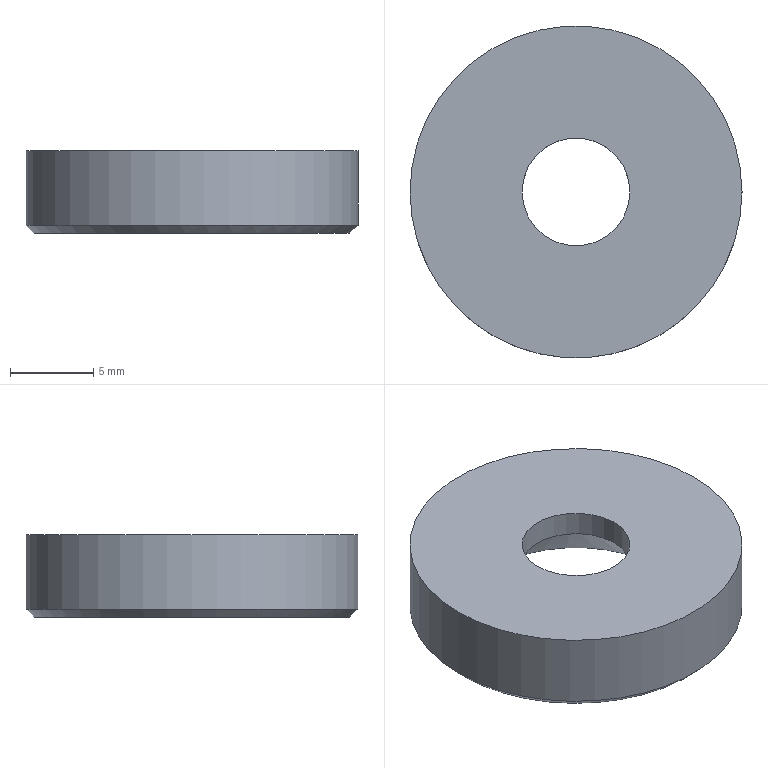Part | STEP file | solid 77 | 1 solid | 6 faces | box 20 x 20 x 5 mm | volume 1227 mm3 | plane 2 | cone 2 | cylinder 2 | commonest cylinder face diameters 6.5 x1 20 x1